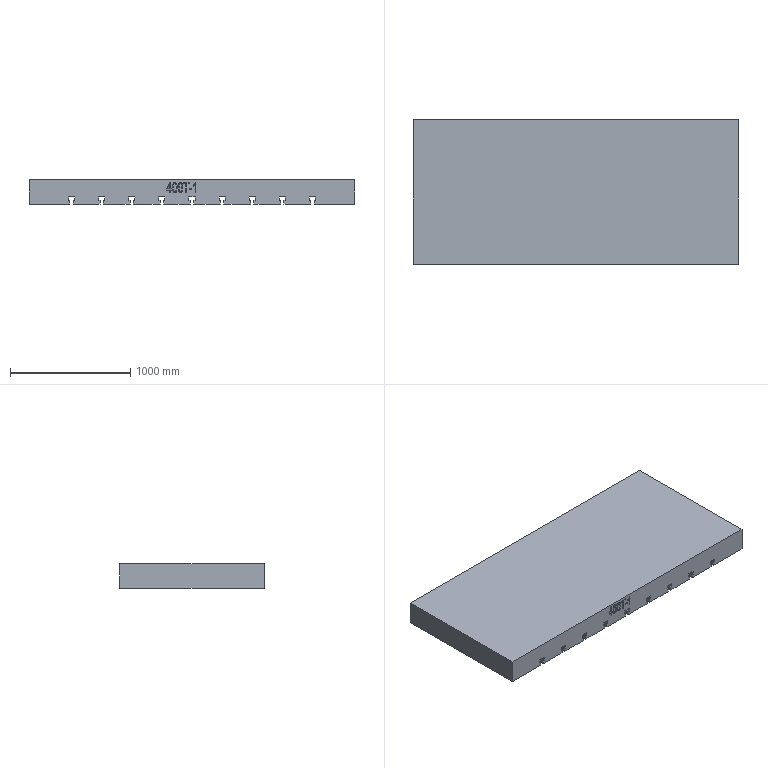Part | NX | features solid 2 | 1 solid | 128 faces | box 2700 x 1200 x 200 mm | volume 622724830 mm3 | plane 118 | spline 10